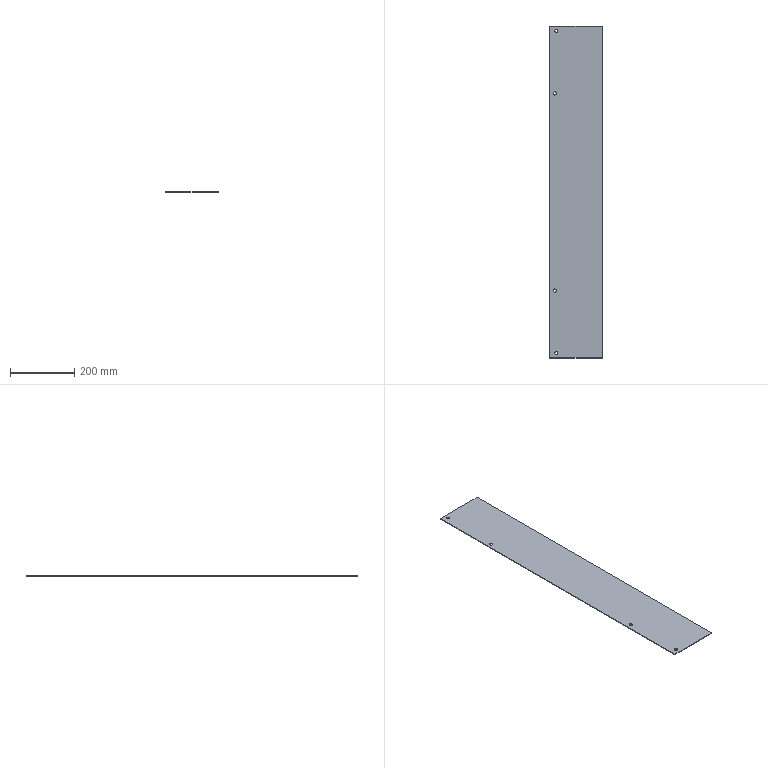Part | STEP file | 1 solid | 14 faces | box 162.5 x 1034 x 2 mm | volume 335422 mm3 | cylinder 8 | plane 6 | commonest cylinder face diameters 10 x8
STEP:
#1=CARTESIAN_POINT('',(0.,0.,0.));
#2=DIRECTION('',(0.,0.,1.));
#3=DIRECTION('',(1.,0.,0.));
#4=AXIS2_PLACEMENT_3D('',#1,#2,#3);
#5=CARTESIAN_POINT('',(-60.73,-722.451,2.));
#6=VERTEX_POINT('',#5);
#7=CARTESIAN_POINT('',(-60.73,-722.451,0.));
#8=VERTEX_POINT('',#7);
#9=CARTESIAN_POINT('',(-60.73,-722.451,2.));
#10=DIRECTION('',(0.,0.,-1.));
#11=VECTOR('',#10,1.);
#12=LINE('',#9,#11);
#13=CARTESIAN_POINT('',(-55.73,-722.451,2.));
#14=DIRECTION('',(0.,0.,-1.));
#15=DIRECTION('',(-1.,0.,0.));
#16=AXIS2_PLACEMENT_3D('',#13,#14,#15);
#17=CYLINDRICAL_SURFACE('',#16,5.);
#18=CARTESIAN_POINT('',(6.283,0.));
#19=DIRECTION('',(0.,1.));
#20=VECTOR('',#19,1.);
#21=LINE('',#18,#20);
#22=(GEOMETRIC_REPRESENTATION_CONTEXT(2)PARAMETRIC_REPRESENTATION_CONTEXT()REPRESENTATION_CONTEXT('',''));
#23=DEFINITIONAL_REPRESENTATION('',(#21),#22);
#24=PCURVE('',#17,#23);
#25=CARTESIAN_POINT('',(-55.73,-722.451,2.));
#26=DIRECTION('',(0.,0.,-1.));
#27=DIRECTION('',(-1.,0.,0.));
#28=AXIS2_PLACEMENT_3D('',#25,#26,#27);
#29=CYLINDRICAL_SURFACE('',#28,5.);
#30=CARTESIAN_POINT('',(0.,0.));
#31=DIRECTION('',(0.,1.));
#32=VECTOR('',#31,1.);
#33=LINE('',#30,#32);
#34=(GEOMETRIC_REPRESENTATION_CONTEXT(2)PARAMETRIC_REPRESENTATION_CONTEXT()REPRESENTATION_CONTEXT('',''));
#35=DEFINITIONAL_REPRESENTATION('',(#33),#34);
#36=PCURVE('',#29,#35);
#37=SURFACE_CURVE('',#12,(#24,#36),.PCURVE_S1.);
#38=EDGE_CURVE('',#6,#8,#37,.T.);
#39=ORIENTED_EDGE('',*,*,#38,.T.);
#40=CARTESIAN_POINT('',(-50.73,-722.451,0.));
#41=VERTEX_POINT('',#40);
#42=CARTESIAN_POINT('',(-55.73,-722.451,0.));
#43=DIRECTION('',(0.,0.,-1.));
#44=DIRECTION('',(-1.,0.,0.));
#45=AXIS2_PLACEMENT_3D('',#42,#43,#44);
#46=CIRCLE('',#45,5.);
#47=CARTESIAN_POINT('',(0.,2.));
#48=DIRECTION('',(1.,0.));
#49=VECTOR('',#48,1.);
#50=LINE('',#47,#49);
#51=(GEOMETRIC_REPRESENTATION_CONTEXT(2)PARAMETRIC_REPRESENTATION_CONTEXT()REPRESENTATION_CONTEXT('',''));
#52=DEFINITIONAL_REPRESENTATION('',(#50),#51);
#53=PCURVE('',#17,#52);
#54=CARTESIAN_POINT('',(10.52,-415.451,0.));
#55=DIRECTION('',(0.,0.,1.));
#56=DIRECTION('',(1.,0.,0.));
#57=AXIS2_PLACEMENT_3D('',#54,#55,#56);
#58=PLANE('',#57);
#59=CARTESIAN_POINT('',(-71.25,-307.));
#60=CARTESIAN_POINT('',(-71.25,-298.34));
#61=CARTESIAN_POINT('',(-63.75,-302.67));
#62=CARTESIAN_POINT('',(-56.25,-307.));
#63=CARTESIAN_POINT('',(-63.75,-311.33));
#64=CARTESIAN_POINT('',(-71.25,-315.66));
#65=CARTESIAN_POINT('',(-71.25,-307.));
#66=(BOUNDED_CURVE()B_SPLINE_CURVE(2,(#59,#60,#61,#62,#63,#64,#65),.UNSPECIFIED.,.T.,.F.)B_SPLINE_CURVE_WITH_KNOTS((1,2,2,2,2,1),(-2.094,0.,2.094,4.189,6.283,8.378),.UNSPECIFIED.)CURVE()GEOMETRIC_REPRESENTATION_ITEM()RATIONAL_B_SPLINE_CURVE((1.,0.5,1.,0.5,1.,0.5,1.))REPRESENTATION_ITEM(''));
#67=(GEOMETRIC_REPRESENTATION_CONTEXT(2)PARAMETRIC_REPRESENTATION_CONTEXT()REPRESENTATION_CONTEXT('',''));
#68=DEFINITIONAL_REPRESENTATION('',(#66),#67);
#69=PCURVE('',#58,#68);
#70=SURFACE_CURVE('',#46,(#53,#69),.PCURVE_S1.);
#71=EDGE_CURVE('',#41,#8,#70,.T.);
#72=ORIENTED_EDGE('',*,*,#71,.F.);
#73=CARTESIAN_POINT('',(-50.73,-722.451,2.));
#74=VERTEX_POINT('',#73);
#75=CARTESIAN_POINT('',(-50.73,-722.451,2.));
#76=DIRECTION('',(0.,0.,-1.));
#77=VECTOR('',#76,1.);
#78=LINE('',#75,#77);
#79=CARTESIAN_POINT('',(3.142,0.));
#80=DIRECTION('',(0.,1.));
#81=VECTOR('',#80,1.);
#82=LINE('',#79,#81);
#83=(GEOMETRIC_REPRESENTATION_CONTEXT(2)PARAMETRIC_REPRESENTATION_CONTEXT()REPRESENTATION_CONTEXT('',''));
#84=DEFINITIONAL_REPRESENTATION('',(#82),#83);
#85=PCURVE('',#17,#84);
#86=CARTESIAN_POINT('',(3.142,0.));
#87=DIRECTION('',(0.,1.));
#88=VECTOR('',#87,1.);
#89=LINE('',#86,#88);
#90=(GEOMETRIC_REPRESENTATION_CONTEXT(2)PARAMETRIC_REPRESENTATION_CONTEXT()REPRESENTATION_CONTEXT('',''));
#91=DEFINITIONAL_REPRESENTATION('',(#89),#90);
#92=PCURVE('',#29,#91);
#93=SURFACE_CURVE('',#78,(#85,#92),.PCURVE_S1.);
#94=EDGE_CURVE('',#74,#41,#93,.T.);
#95=ORIENTED_EDGE('',*,*,#94,.F.);
#96=CARTESIAN_POINT('',(-55.73,-722.451,2.));
#97=DIRECTION('',(0.,0.,-1.));
#98=DIRECTION('',(-1.,0.,0.));
#99=AXIS2_PLACEMENT_3D('',#96,#97,#98);
#100=CIRCLE('',#99,5.);
#101=CARTESIAN_POINT('',(0.,0.));
#102=DIRECTION('',(1.,0.));
#103=VECTOR('',#102,1.);
#104=LINE('',#101,#103);
#105=(GEOMETRIC_REPRESENTATION_CONTEXT(2)PARAMETRIC_REPRESENTATION_CONTEXT()REPRESENTATION_CONTEXT('',''));
#106=DEFINITIONAL_REPRESENTATION('',(#104),#105);
#107=PCURVE('',#17,#106);
#108=CARTESIAN_POINT('',(10.52,-415.451,2.));
#109=DIRECTION('',(0.,0.,1.));
#110=DIRECTION('',(1.,0.,0.));
#111=AXIS2_PLACEMENT_3D('',#108,#109,#110);
#112=PLANE('',#111);
#113=CARTESIAN_POINT('',(-71.25,-307.));
#114=CARTESIAN_POINT('',(-71.25,-298.34));
#115=CARTESIAN_POINT('',(-63.75,-302.67));
#116=CARTESIAN_POINT('',(-56.25,-307.));
#117=CARTESIAN_POINT('',(-63.75,-311.33));
#118=CARTESIAN_POINT('',(-71.25,-315.66));
#119=CARTESIAN_POINT('',(-71.25,-307.));
#120=(BOUNDED_CURVE()B_SPLINE_CURVE(2,(#113,#114,#115,#116,#117,#118,#119),.UNSPECIFIED.,.T.,.F.)B_SPLINE_CURVE_WITH_KNOTS((1,2,2,2,2,1),(-2.094,0.,2.094,4.189,6.283,8.378),.UNSPECIFIED.)CURVE()GEOMETRIC_REPRESENTATION_ITEM()RATIONAL_B_SPLINE_CURVE((1.,0.5,1.,0.5,1.,0.5,1.))REPRESENTATION_ITEM(''));
#121=(GEOMETRIC_REPRESENTATION_CONTEXT(2)PARAMETRIC_REPRESENTATION_CONTEXT()REPRESENTATION_CONTEXT('',''));
#122=DEFINITIONAL_REPRESENTATION('',(#120),#121);
#123=PCURVE('',#112,#122);
#124=SURFACE_CURVE('',#100,(#107,#123),.PCURVE_S1.);
#125=EDGE_CURVE('',#74,#6,#124,.T.);
#126=ORIENTED_EDGE('',*,*,#125,.T.);
#127=EDGE_LOOP('',(#39,#72,#95,#126));
#128=FACE_BOUND('',#127,.F.);
#129=ADVANCED_FACE('',(#128),#17,.F.);
#130=CARTESIAN_POINT('',(-60.73,-108.451,2.));
#131=VERTEX_POINT('',#130);
#132=CARTESIAN_POINT('',(-60.73,-108.451,0.));
#133=VERTEX_POINT('',#132);
#134=CARTESIAN_POINT('',(-60.73,-108.451,2.));
#135=DIRECTION('',(0.,0.,-1.));
#136=VECTOR('',#135,1.);
#137=LINE('',#134,#136);
#138=CARTESIAN_POINT('',(-55.73,-108.451,2.));
#139=DIRECTION('',(0.,0.,-1.));
#140=DIRECTION('',(-1.,0.,0.));
#141=AXIS2_PLACEMENT_3D('',#138,#139,#140);
#142=CYLINDRICAL_SURFACE('',#141,5.);
#143=CARTESIAN_POINT('',(6.283,0.));
#144=DIRECTION('',(0.,1.));
#145=VECTOR('',#144,1.);
#146=LINE('',#143,#145);
#147=(GEOMETRIC_REPRESENTATION_CONTEXT(2)PARAMETRIC_REPRESENTATION_CONTEXT()REPRESENTATION_CONTEXT('',''));
#148=DEFINITIONAL_REPRESENTATION('',(#146),#147);
#149=PCURVE('',#142,#148);
#150=CARTESIAN_POINT('',(-55.73,-108.451,2.));
#151=DIRECTION('',(0.,0.,-1.));
#152=DIRECTION('',(-1.,0.,0.));
#153=AXIS2_PLACEMENT_3D('',#150,#151,#152);
#154=CYLINDRICAL_SURFACE('',#153,5.);
#155=CARTESIAN_POINT('',(0.,0.));
#156=DIRECTION('',(0.,1.));
#157=VECTOR('',#156,1.);
#158=LINE('',#155,#157);
#159=(GEOMETRIC_REPRESENTATION_CONTEXT(2)PARAMETRIC_REPRESENTATION_CONTEXT()REPRESENTATION_CONTEXT('',''));
#160=DEFINITIONAL_REPRESENTATION('',(#158),#159);
#161=PCURVE('',#154,#160);
#162=SURFACE_CURVE('',#137,(#149,#161),.PCURVE_S1.);
#163=EDGE_CURVE('',#131,#133,#162,.T.);
#164=ORIENTED_EDGE('',*,*,#163,.T.);
#165=CARTESIAN_POINT('',(-50.73,-108.451,0.));
#166=VERTEX_POINT('',#165);
#167=CARTESIAN_POINT('',(-55.73,-108.451,0.));
#168=DIRECTION('',(0.,0.,-1.));
#169=DIRECTION('',(-1.,0.,0.));
#170=AXIS2_PLACEMENT_3D('',#167,#168,#169);
#171=CIRCLE('',#170,5.);
#172=CARTESIAN_POINT('',(0.,2.));
#173=DIRECTION('',(1.,0.));
#174=VECTOR('',#173,1.);
#175=LINE('',#172,#174);
#176=(GEOMETRIC_REPRESENTATION_CONTEXT(2)PARAMETRIC_REPRESENTATION_CONTEXT()REPRESENTATION_CONTEXT('',''));
#177=DEFINITIONAL_REPRESENTATION('',(#175),#176);
#178=PCURVE('',#142,#177);
#179=CARTESIAN_POINT('',(-71.25,307.));
#180=CARTESIAN_POINT('',(-71.25,315.66));
#181=CARTESIAN_POINT('',(-63.75,311.33));
#182=CARTESIAN_POINT('',(-56.25,307.));
#183=CARTESIAN_POINT('',(-63.75,302.67));
#184=CARTESIAN_POINT('',(-71.25,298.34));
#185=CARTESIAN_POINT('',(-71.25,307.));
#186=(BOUNDED_CURVE()B_SPLINE_CURVE(2,(#179,#180,#181,#182,#183,#184,#185),.UNSPECIFIED.,.T.,.F.)B_SPLINE_CURVE_WITH_KNOTS((1,2,2,2,2,1),(-2.094,0.,2.094,4.189,6.283,8.378),.UNSPECIFIED.)CURVE()GEOMETRIC_REPRESENTATION_ITEM()RATIONAL_B_SPLINE_CURVE((1.,0.5,1.,0.5,1.,0.5,1.))REPRESENTATION_ITEM(''));
#187=(GEOMETRIC_REPRESENTATION_CONTEXT(2)PARAMETRIC_REPRESENTATION_CONTEXT()REPRESENTATION_CONTEXT('',''));
#188=DEFINITIONAL_REPRESENTATION('',(#186),#187);
#189=PCURVE('',#58,#188);
#190=SURFACE_CURVE('',#171,(#178,#189),.PCURVE_S1.);
#191=EDGE_CURVE('',#166,#133,#190,.T.);
#192=ORIENTED_EDGE('',*,*,#191,.F.);
#193=CARTESIAN_POINT('',(-50.73,-108.451,2.));
#194=VERTEX_POINT('',#193);
#195=CARTESIAN_POINT('',(-50.73,-108.451,2.));
#196=DIRECTION('',(0.,0.,-1.));
#197=VECTOR('',#196,1.);
#198=LINE('',#195,#197);
#199=CARTESIAN_POINT('',(3.142,0.));
#200=DIRECTION('',(0.,1.));
#201=VECTOR('',#200,1.);
#202=LINE('',#199,#201);
#203=(GEOMETRIC_REPRESENTATION_CONTEXT(2)PARAMETRIC_REPRESENTATION_CONTEXT()REPRESENTATION_CONTEXT('',''));
#204=DEFINITIONAL_REPRESENTATION('',(#202),#203);
#205=PCURVE('',#142,#204);
#206=CARTESIAN_POINT('',(3.142,0.));
#207=DIRECTION('',(0.,1.));
#208=VECTOR('',#207,1.);
#209=LINE('',#206,#208);
#210=(GEOMETRIC_REPRESENTATION_CONTEXT(2)PARAMETRIC_REPRESENTATION_CONTEXT()REPRESENTATION_CONTEXT('',''));
#211=DEFINITIONAL_REPRESENTATION('',(#209),#210);
#212=PCURVE('',#154,#211);
#213=SURFACE_CURVE('',#198,(#205,#212),.PCURVE_S1.);
#214=EDGE_CURVE('',#194,#166,#213,.T.);
#215=ORIENTED_EDGE('',*,*,#214,.F.);
#216=CARTESIAN_POINT('',(-55.73,-108.451,2.));
#217=DIRECTION('',(0.,0.,-1.));
#218=DIRECTION('',(-1.,0.,0.));
#219=AXIS2_PLACEMENT_3D('',#216,#217,#218);
#220=CIRCLE('',#219,5.);
#221=CARTESIAN_POINT('',(0.,0.));
#222=DIRECTION('',(1.,0.));
#223=VECTOR('',#222,1.);
#224=LINE('',#221,#223);
#225=(GEOMETRIC_REPRESENTATION_CONTEXT(2)PARAMETRIC_REPRESENTATION_CONTEXT()REPRESENTATION_CONTEXT('',''));
#226=DEFINITIONAL_REPRESENTATION('',(#224),#225);
#227=PCURVE('',#142,#226);
#228=CARTESIAN_POINT('',(-71.25,307.));
#229=CARTESIAN_POINT('',(-71.25,315.66));
#230=CARTESIAN_POINT('',(-63.75,311.33));
#231=CARTESIAN_POINT('',(-56.25,307.));
#232=CARTESIAN_POINT('',(-63.75,302.67));
#233=CARTESIAN_POINT('',(-71.25,298.34));
#234=CARTESIAN_POINT('',(-71.25,307.));
#235=(BOUNDED_CURVE()B_SPLINE_CURVE(2,(#228,#229,#230,#231,#232,#233,#234),.UNSPECIFIED.,.T.,.F.)B_SPLINE_CURVE_WITH_KNOTS((1,2,2,2,2,1),(-2.094,0.,2.094,4.189,6.283,8.378),.UNSPECIFIED.)CURVE()GEOMETRIC_REPRESENTATION_ITEM()RATIONAL_B_SPLINE_CURVE((1.,0.5,1.,0.5,1.,0.5,1.))REPRESENTATION_ITEM(''));
#236=(GEOMETRIC_REPRESENTATION_CONTEXT(2)PARAMETRIC_REPRESENTATION_CONTEXT()REPRESENTATION_CONTEXT('',''));
#237=DEFINITIONAL_REPRESENTATION('',(#235),#236);
#238=PCURVE('',#112,#237);
#239=SURFACE_CURVE('',#220,(#227,#238),.PCURVE_S1.);
#240=EDGE_CURVE('',#194,#131,#239,.T.);
#241=ORIENTED_EDGE('',*,*,#240,.T.);
#242=EDGE_LOOP('',(#164,#192,#215,#241));
#243=FACE_BOUND('',#242,.F.);
#244=ADVANCED_FACE('',(#243),#142,.F.);
#245=CARTESIAN_POINT('',(-55.73,-917.451,2.));
#246=VERTEX_POINT('',#245);
#247=CARTESIAN_POINT('',(-55.73,-917.451,0.));
#248=VERTEX_POINT('',#247);
#249=CARTESIAN_POINT('',(-55.73,-917.451,2.));
#250=DIRECTION('',(0.,0.,-1.));
#251=VECTOR('',#250,1.);
#252=LINE('',#249,#251);
#253=CARTESIAN_POINT('',(-50.73,-917.451,2.));
#254=DIRECTION('',(0.,0.,-1.));
#255=DIRECTION('',(-1.,0.,0.));
#256=AXIS2_PLACEMENT_3D('',#253,#254,#255);
#257=CYLINDRICAL_SURFACE('',#256,5.);
#258=CARTESIAN_POINT('',(6.283,0.));
#259=DIRECTION('',(0.,1.));
#260=VECTOR('',#259,1.);
#261=LINE('',#258,#260);
#262=(GEOMETRIC_REPRESENTATION_CONTEXT(2)PARAMETRIC_REPRESENTATION_CONTEXT()REPRESENTATION_CONTEXT('',''));
#263=DEFINITIONAL_REPRESENTATION('',(#261),#262);
#264=PCURVE('',#257,#263);
#265=CARTESIAN_POINT('',(-50.73,-917.451,2.));
#266=DIRECTION('',(0.,0.,-1.));
#267=DIRECTION('',(-1.,0.,0.));
#268=AXIS2_PLACEMENT_3D('',#265,#266,#267);
#269=CYLINDRICAL_SURFACE('',#268,5.);
#270=CARTESIAN_POINT('',(0.,0.));
#271=DIRECTION('',(0.,1.));
#272=VECTOR('',#271,1.);
#273=LINE('',#270,#272);
#274=(GEOMETRIC_REPRESENTATION_CONTEXT(2)PARAMETRIC_REPRESENTATION_CONTEXT()REPRESENTATION_CONTEXT('',''));
#275=DEFINITIONAL_REPRESENTATION('',(#273),#274);
#276=PCURVE('',#269,#275);
#277=SURFACE_CURVE('',#252,(#264,#276),.PCURVE_S1.);
#278=EDGE_CURVE('',#246,#248,#277,.T.);
#279=ORIENTED_EDGE('',*,*,#278,.T.);
#280=CARTESIAN_POINT('',(-45.73,-917.451,0.));
#281=VERTEX_POINT('',#280);
#282=CARTESIAN_POINT('',(-50.73,-917.451,0.));
#283=DIRECTION('',(0.,0.,-1.));
#284=DIRECTION('',(-1.,0.,0.));
#285=AXIS2_PLACEMENT_3D('',#282,#283,#284);
#286=CIRCLE('',#285,5.);
#287=CARTESIAN_POINT('',(0.,2.));
#288=DIRECTION('',(1.,0.));
#289=VECTOR('',#288,1.);
#290=LINE('',#287,#289);
#291=(GEOMETRIC_REPRESENTATION_CONTEXT(2)PARAMETRIC_REPRESENTATION_CONTEXT()REPRESENTATION_CONTEXT('',''));
#292=DEFINITIONAL_REPRESENTATION('',(#290),#291);
#293=PCURVE('',#257,#292);
#294=CARTESIAN_POINT('',(-66.25,-502.));
#295=CARTESIAN_POINT('',(-66.25,-493.34));
#296=CARTESIAN_POINT('',(-58.75,-497.67));
#297=CARTESIAN_POINT('',(-51.25,-502.));
#298=CARTESIAN_POINT('',(-58.75,-506.33));
#299=CARTESIAN_POINT('',(-66.25,-510.66));
#300=CARTESIAN_POINT('',(-66.25,-502.));
#301=(BOUNDED_CURVE()B_SPLINE_CURVE(2,(#294,#295,#296,#297,#298,#299,#300),.UNSPECIFIED.,.T.,.F.)B_SPLINE_CURVE_WITH_KNOTS((1,2,2,2,2,1),(-2.094,0.,2.094,4.189,6.283,8.378),.UNSPECIFIED.)CURVE()GEOMETRIC_REPRESENTATION_ITEM()RATIONAL_B_SPLINE_CURVE((1.,0.5,1.,0.5,1.,0.5,1.))REPRESENTATION_ITEM(''));
#302=(GEOMETRIC_REPRESENTATION_CONTEXT(2)PARAMETRIC_REPRESENTATION_CONTEXT()REPRESENTATION_CONTEXT('',''));
#303=DEFINITIONAL_REPRESENTATION('',(#301),#302);
#304=PCURVE('',#58,#303);
#305=SURFACE_CURVE('',#286,(#293,#304),.PCURVE_S1.);
#306=EDGE_CURVE('',#281,#248,#305,.T.);
#307=ORIENTED_EDGE('',*,*,#306,.F.);
#308=CARTESIAN_POINT('',(-45.73,-917.451,2.));
#309=VERTEX_POINT('',#308);
#310=CARTESIAN_POINT('',(-45.73,-917.451,2.));
#311=DIRECTION('',(0.,0.,-1.));
#312=VECTOR('',#311,1.);
#313=LINE('',#310,#312);
#314=CARTESIAN_POINT('',(3.142,0.));
#315=DIRECTION('',(0.,1.));
#316=VECTOR('',#315,1.);
#317=LINE('',#314,#316);
#318=(GEOMETRIC_REPRESENTATION_CONTEXT(2)PARAMETRIC_REPRESENTATION_CONTEXT()REPRESENTATION_CONTEXT('',''));
#319=DEFINITIONAL_REPRESENTATION('',(#317),#318);
#320=PCURVE('',#257,#319);
#321=CARTESIAN_POINT('',(3.142,0.));
#322=DIRECTION('',(0.,1.));
#323=VECTOR('',#322,1.);
#324=LINE('',#321,#323);
#325=(GEOMETRIC_REPRESENTATION_CONTEXT(2)PARAMETRIC_REPRESENTATION_CONTEXT()REPRESENTATION_CONTEXT('',''));
#326=DEFINITIONAL_REPRESENTATION('',(#324),#325);
#327=PCURVE('',#269,#326);
#328=SURFACE_CURVE('',#313,(#320,#327),.PCURVE_S1.);
#329=EDGE_CURVE('',#309,#281,#328,.T.);
#330=ORIENTED_EDGE('',*,*,#329,.F.);
#331=CARTESIAN_POINT('',(-50.73,-917.451,2.));
#332=DIRECTION('',(0.,0.,-1.));
#333=DIRECTION('',(-1.,0.,0.));
#334=AXIS2_PLACEMENT_3D('',#331,#332,#333);
#335=CIRCLE('',#334,5.);
#336=CARTESIAN_POINT('',(0.,0.));
#337=DIRECTION('',(1.,0.));
#338=VECTOR('',#337,1.);
#339=LINE('',#336,#338);
#340=(GEOMETRIC_REPRESENTATION_CONTEXT(2)PARAMETRIC_REPRESENTATION_CONTEXT()REPRESENTATION_CONTEXT('',''));
#341=DEFINITIONAL_REPRESENTATION('',(#339),#340);
#342=PCURVE('',#257,#341);
#343=CARTESIAN_POINT('',(-66.25,-502.));
#344=CARTESIAN_POINT('',(-66.25,-493.34));
#345=CARTESIAN_POINT('',(-58.75,-497.67));
#346=CARTESIAN_POINT('',(-51.25,-502.));
#347=CARTESIAN_POINT('',(-58.75,-506.33));
#348=CARTESIAN_POINT('',(-66.25,-510.66));
#349=CARTESIAN_POINT('',(-66.25,-502.));
#350=(BOUNDED_CURVE()B_SPLINE_CURVE(2,(#343,#344,#345,#346,#347,#348,#349),.UNSPECIFIED.,.T.,.F.)B_SPLINE_CURVE_WITH_KNOTS((1,2,2,2,2,1),(-2.094,0.,2.094,4.189,6.283,8.378),.UNSPECIFIED.)CURVE()GEOMETRIC_REPRESENTATION_ITEM()RATIONAL_B_SPLINE_CURVE((1.,0.5,1.,0.5,1.,0.5,1.))REPRESENTATION_ITEM(''));
#351=(GEOMETRIC_REPRESENTATION_CONTEXT(2)PARAMETRIC_REPRESENTATION_CONTEXT()REPRESENTATION_CONTEXT('',''));
#352=DEFINITIONAL_REPRESENTATION('',(#350),#351);
#353=PCURVE('',#112,#352);
#354=SURFACE_CURVE('',#335,(#342,#353),.PCURVE_S1.);
#355=EDGE_CURVE('',#309,#246,#354,.T.);
#356=ORIENTED_EDGE('',*,*,#355,.T.);
#357=EDGE_LOOP('',(#279,#307,#330,#356));
#358=FACE_BOUND('',#357,.F.);
#359=ADVANCED_FACE('',(#358),#257,.F.);
#360=CARTESIAN_POINT('',(-55.73,86.549,2.));
#361=VERTEX_POINT('',#360);
#362=CARTESIAN_POINT('',(-55.73,86.549,0.));
#363=VERTEX_POINT('',#362);
#364=CARTESIAN_POINT('',(-55.73,86.549,2.));
#365=DIRECTION('',(0.,0.,-1.));
#366=VECTOR('',#365,1.);
#367=LINE('',#364,#366);
#368=CARTESIAN_POINT('',(-50.73,86.549,2.));
#369=DIRECTION('',(0.,0.,-1.));
#370=DIRECTION('',(-1.,0.,0.));
#371=AXIS2_PLACEMENT_3D('',#368,#369,#370);
#372=CYLINDRICAL_SURFACE('',#371,5.);
#373=CARTESIAN_POINT('',(6.283,0.));
#374=DIRECTION('',(0.,1.));
#375=VECTOR('',#374,1.);
#376=LINE('',#373,#375);
#377=(GEOMETRIC_REPRESENTATION_CONTEXT(2)PARAMETRIC_REPRESENTATION_CONTEXT()REPRESENTATION_CONTEXT('',''));
#378=DEFINITIONAL_REPRESENTATION('',(#376),#377);
#379=PCURVE('',#372,#378);
#380=CARTESIAN_POINT('',(-50.73,86.549,2.));
#381=DIRECTION('',(0.,0.,-1.));
#382=DIRECTION('',(-1.,0.,0.));
#383=AXIS2_PLACEMENT_3D('',#380,#381,#382);
#384=CYLINDRICAL_SURFACE('',#383,5.);
#385=CARTESIAN_POINT('',(0.,0.));
#386=DIRECTION('',(0.,1.));
#387=VECTOR('',#386,1.);
#388=LINE('',#385,#387);
#389=(GEOMETRIC_REPRESENTATION_CONTEXT(2)PARAMETRIC_REPRESENTATION_CONTEXT()REPRESENTATION_CONTEXT('',''));
#390=DEFINITIONAL_REPRESENTATION('',(#388),#389);
#391=PCURVE('',#384,#390);
#392=SURFACE_CURVE('',#367,(#379,#391),.PCURVE_S1.);
#393=EDGE_CURVE('',#361,#363,#392,.T.);
#394=ORIENTED_EDGE('',*,*,#393,.T.);
#395=CARTESIAN_POINT('',(-45.73,86.549,0.));
#396=VERTEX_POINT('',#395);
#397=CARTESIAN_POINT('',(-50.73,86.549,0.));
#398=DIRECTION('',(0.,0.,-1.));
#399=DIRECTION('',(-1.,0.,0.));
#400=AXIS2_PLACEMENT_3D('',#397,#398,#399);
#401=CIRCLE('',#400,5.);
#402=CARTESIAN_POINT('',(0.,2.));
#403=DIRECTION('',(1.,0.));
#404=VECTOR('',#403,1.);
#405=LINE('',#402,#404);
#406=(GEOMETRIC_REPRESENTATION_CONTEXT(2)PARAMETRIC_REPRESENTATION_CONTEXT()REPRESENTATION_CONTEXT('',''));
#407=DEFINITIONAL_REPRESENTATION('',(#405),#406);
#408=PCURVE('',#372,#407);
#409=CARTESIAN_POINT('',(-66.25,502.));
#410=CARTESIAN_POINT('',(-66.25,510.66));
#411=CARTESIAN_POINT('',(-58.75,506.33));
#412=CARTESIAN_POINT('',(-51.25,502.));
#413=CARTESIAN_POINT('',(-58.75,497.67));
#414=CARTESIAN_POINT('',(-66.25,493.34));
#415=CARTESIAN_POINT('',(-66.25,502.));
#416=(BOUNDED_CURVE()B_SPLINE_CURVE(2,(#409,#410,#411,#412,#413,#414,#415),.UNSPECIFIED.,.T.,.F.)B_SPLINE_CURVE_WITH_KNOTS((1,2,2,2,2,1),(-2.094,0.,2.094,4.189,6.283,8.378),.UNSPECIFIED.)CURVE()GEOMETRIC_REPRESENTATION_ITEM()RATIONAL_B_SPLINE_CURVE((1.,0.5,1.,0.5,1.,0.5,1.))REPRESENTATION_ITEM(''));
#417=(GEOMETRIC_REPRESENTATION_CONTEXT(2)PARAMETRIC_REPRESENTATION_CONTEXT()REPRESENTATION_CONTEXT('',''));
#418=DEFINITIONAL_REPRESENTATION('',(#416),#417);
#419=PCURVE('',#58,#418);
#420=SURFACE_CURVE('',#401,(#408,#419),.PCURVE_S1.);
#421=EDGE_CURVE('',#396,#363,#420,.T.);
#422=ORIENTED_EDGE('',*,*,#421,.F.);
#423=CARTESIAN_POINT('',(-45.73,86.549,2.));
#424=VERTEX_POINT('',#423);
#425=CARTESIAN_POINT('',(-45.73,86.549,2.));
#426=DIRECTION('',(0.,0.,-1.));
#427=VECTOR('',#426,1.);
#428=LINE('',#425,#427);
#429=CARTESIAN_POINT('',(3.142,0.));
#430=DIRECTION('',(0.,1.));
#431=VECTOR('',#430,1.);
#432=LINE('',#429,#431);
#433=(GEOMETRIC_REPRESENTATION_CONTEXT(2)PARAMETRIC_REPRESENTATION_CONTEXT()REPRESENTATION_CONTEXT('',''));
#434=DEFINITIONAL_REPRESENTATION('',(#432),#433);
#435=PCURVE('',#372,#434);
#436=CARTESIAN_POINT('',(3.142,0.));
#437=DIRECTION('',(0.,1.));
#438=VECTOR('',#437,1.);
#439=LINE('',#436,#438);
#440=(GEOMETRIC_REPRESENTATION_CONTEXT(2)PARAMETRIC_REPRESENTATION_CONTEXT()REPRESENTATION_CONTEXT('',''));
#441=DEFINITIONAL_REPRESENTATION('',(#439),#440);
#442=PCURVE('',#384,#441);
#443=SURFACE_CURVE('',#428,(#435,#442),.PCURVE_S1.);
#444=EDGE_CURVE('',#424,#396,#443,.T.);
#445=ORIENTED_EDGE('',*,*,#444,.F.);
#446=CARTESIAN_POINT('',(-50.73,86.549,2.));
#447=DIRECTION('',(0.,0.,-1.));
#448=DIRECTION('',(-1.,0.,0.));
#449=AXIS2_PLACEMENT_3D('',#446,#447,#448);
#450=CIRCLE('',#449,5.);
#451=CARTESIAN_POINT('',(0.,0.));
#452=DIRECTION('',(1.,0.));
#453=VECTOR('',#452,1.);
#454=LINE('',#451,#453);
#455=(GEOMETRIC_REPRESENTATION_CONTEXT(2)PARAMETRIC_REPRESENTATION_CONTEXT()REPRESENTATION_CONTEXT('',''));
#456=DEFINITIONAL_REPRESENTATION('',(#454),#455);
#457=PCURVE('',#372,#456);
#458=CARTESIAN_POINT('',(-66.25,502.));
#459=CARTESIAN_POINT('',(-66.25,510.66));
#460=CARTESIAN_POINT('',(-58.75,506.33));
#461=CARTESIAN_POINT('',(-51.25,502.));
#462=CARTESIAN_POINT('',(-58.75,497.67));
#463=CARTESIAN_POINT('',(-66.25,493.34));
#464=CARTESIAN_POINT('',(-66.25,502.));
#465=(BOUNDED_CURVE()B_SPLINE_CURVE(2,(#458,#459,#460,#461,#462,#463,#464),.UNSPECIFIED.,.T.,.F.)B_SPLINE_CURVE_WITH_KNOTS((1,2,2,2,2,1),(-2.094,0.,2.094,4.189,6.283,8.378),.UNSPECIFIED.)CURVE()GEOMETRIC_REPRESENTATION_ITEM()RATIONAL_B_SPLINE_CURVE((1.,0.5,1.,0.5,1.,0.5,1.))REPRESENTATION_ITEM(''));
#466=(GEOMETRIC_REPRESENTATION_CONTEXT(2)PARAMETRIC_REPRESENTATION_CONTEXT()REPRESENTATION_CONTEXT('',''));
#467=DEFINITIONAL_REPRESENTATION('',(#465),#466);
#468=PCURVE('',#112,#467);
#469=SURFACE_CURVE('',#450,(#457,#468),.PCURVE_S1.);
#470=EDGE_CURVE('',#424,#361,#469,.T.);
#471=ORIENTED_EDGE('',*,*,#470,.T.);
#472=EDGE_LOOP('',(#394,#422,#445,#471));
#473=FACE_BOUND('',#472,.F.);
#474=ADVANCED_FACE('',(#473),#372,.F.);
#475=CARTESIAN_POINT('',(91.77,-932.451,0.));
#476=VERTEX_POINT('',#475);
#477=CARTESIAN_POINT('',(91.77,101.549,0.));
#478=VERTEX_POINT('',#477);
#479=CARTESIAN_POINT('',(91.77,-415.451,0.));
#480=DIRECTION('',(0.,1.,0.));
#481=VECTOR('',#480,1.);
#482=LINE('',#479,#481);
#483=CARTESIAN_POINT('',(81.25,0.));
#484=DIRECTION('',(0.,1.));
#485=VECTOR('',#484,1.);
#486=LINE('',#483,#485);
#487=(GEOMETRIC_REPRESENTATION_CONTEXT(2)PARAMETRIC_REPRESENTATION_CONTEXT()REPRESENTATION_CONTEXT('',''));
#488=DEFINITIONAL_REPRESENTATION('',(#486),#487);
#489=PCURVE('',#58,#488);
#490=CARTESIAN_POINT('',(91.77,-932.451,0.));
#491=DIRECTION('',(1.,0.,0.));
#492=DIRECTION('',(0.,1.,0.));
#493=AXIS2_PLACEMENT_3D('',#490,#491,#492);
#494=PLANE('',#493);
#495=CARTESIAN_POINT('',(517.,0.));
#496=DIRECTION('',(1.,0.));
#497=VECTOR('',#496,1.);
#498=LINE('',#495,#497);
#499=(GEOMETRIC_REPRESENTATION_CONTEXT(2)PARAMETRIC_REPRESENTATION_CONTEXT()REPRESENTATION_CONTEXT('',''));
#500=DEFINITIONAL_REPRESENTATION('',(#498),#499);
#501=PCURVE('',#494,#500);
#502=SURFACE_CURVE('',#482,(#489,#501),.PCURVE_S1.);
#503=EDGE_CURVE('',#476,#478,#502,.T.);
#504=ORIENTED_EDGE('',*,*,#503,.F.);
#505=CARTESIAN_POINT('',(-70.73,-932.451,0.));
#506=VERTEX_POINT('',#505);
#507=CARTESIAN_POINT('',(10.52,-932.451,0.));
#508=DIRECTION('',(1.,0.,0.));
#509=VECTOR('',#508,1.);
#510=LINE('',#507,#509);
#511=CARTESIAN_POINT('',(0.,-517.));
#512=DIRECTION('',(1.,0.));
#513=VECTOR('',#512,1.);
#514=LINE('',#511,#513);
#515=(GEOMETRIC_REPRESENTATION_CONTEXT(2)PARAMETRIC_REPRESENTATION_CONTEXT()REPRESENTATION_CONTEXT('',''));
#516=DEFINITIONAL_REPRESENTATION('',(#514),#515);
#517=PCURVE('',#58,#516);
#518=CARTESIAN_POINT('',(-70.73,-932.451,0.));
#519=DIRECTION('',(0.,-1.,0.));
#520=DIRECTION('',(0.,0.,-1.));
#521=AXIS2_PLACEMENT_3D('',#518,#519,#520);
#522=PLANE('',#521);
#523=CARTESIAN_POINT('',(0.,81.25));
#524=DIRECTION('',(0.,1.));
#525=VECTOR('',#524,1.);
#526=LINE('',#523,#525);
#527=(GEOMETRIC_REPRESENTATION_CONTEXT(2)PARAMETRIC_REPRESENTATION_CONTEXT()REPRESENTATION_CONTEXT('',''));
#528=DEFINITIONAL_REPRESENTATION('',(#526),#527);
#529=PCURVE('',#522,#528);
#530=SURFACE_CURVE('',#510,(#517,#529),.PCURVE_S1.);
#531=EDGE_CURVE('',#506,#476,#530,.T.);
#532=ORIENTED_EDGE('',*,*,#531,.F.);
#533=CARTESIAN_POINT('',(-70.73,101.549,0.));
#534=VERTEX_POINT('',#533);
#535=CARTESIAN_POINT('',(-70.73,-415.451,0.));
#536=DIRECTION('',(0.,-1.,0.));
#537=VECTOR('',#536,1.);
#538=LINE('',#535,#537);
#539=CARTESIAN_POINT('',(-81.25,0.));
#540=DIRECTION('',(0.,-1.));
#541=VECTOR('',#540,1.);
#542=LINE('',#539,#541);
#543=(GEOMETRIC_REPRESENTATION_CONTEXT(2)PARAMETRIC_REPRESENTATION_CONTEXT()REPRESENTATION_CONTEXT('',''));
#544=DEFINITIONAL_REPRESENTATION('',(#542),#543);
#545=PCURVE('',#58,#544);
#546=CARTESIAN_POINT('',(-70.73,101.549,0.));
#547=DIRECTION('',(-1.,0.,0.));
#548=DIRECTION('',(0.,-1.,0.));
#549=AXIS2_PLACEMENT_3D('',#546,#547,#548);
#550=PLANE('',#549);
#551=CARTESIAN_POINT('',(517.,0.));
#552=DIRECTION('',(1.,0.));
#553=VECTOR('',#552,1.);
#554=LINE('',#551,#553);
#555=(GEOMETRIC_REPRESENTATION_CONTEXT(2)PARAMETRIC_REPRESENTATION_CONTEXT()REPRESENTATION_CONTEXT('',''));
#556=DEFINITIONAL_REPRESENTATION('',(#554),#555);
#557=PCURVE('',#550,#556);
#558=SURFACE_CURVE('',#538,(#545,#557),.PCURVE_S1.);
#559=EDGE_CURVE('',#534,#506,#558,.T.);
#560=ORIENTED_EDGE('',*,*,#559,.F.);
#561=CARTESIAN_POINT('',(10.52,101.549,0.));
#562=DIRECTION('',(-1.,0.,0.));
#563=VECTOR('',#562,1.);
#564=LINE('',#561,#563);
#565=CARTESIAN_POINT('',(0.,517.));
#566=DIRECTION('',(-1.,0.));
#567=VECTOR('',#566,1.);
#568=LINE('',#565,#567);
#569=(GEOMETRIC_REPRESENTATION_CONTEXT(2)PARAMETRIC_REPRESENTATION_CONTEXT()REPRESENTATION_CONTEXT('',''));
#570=DEFINITIONAL_REPRESENTATION('',(#568),#569);
#571=PCURVE('',#58,#570);
#572=CARTESIAN_POINT('',(91.77,101.549,0.));
#573=DIRECTION('',(0.,1.,0.));
#574=DIRECTION('',(0.,0.,1.));
#575=AXIS2_PLACEMENT_3D('',#572,#573,#574);
#576=PLANE('',#575);
#577=CARTESIAN_POINT('',(0.,-81.25));
#578=DIRECTION('',(0.,-1.));
#579=VECTOR('',#578,1.);
#580=LINE('',#577,#579);
#581=(GEOMETRIC_REPRESENTATION_CONTEXT(2)PARAMETRIC_REPRESENTATION_CONTEXT()REPRESENTATION_CONTEXT('',''));
#582=DEFINITIONAL_REPRESENTATION('',(#580),#581);
#583=PCURVE('',#576,#582);
#584=SURFACE_CURVE('',#564,(#571,#583),.PCURVE_S1.);
#585=EDGE_CURVE('',#478,#534,#584,.T.);
#586=ORIENTED_EDGE('',*,*,#585,.F.);
#587=EDGE_LOOP('',(#504,#532,#560,#586));
#588=FACE_BOUND('',#587,.T.);
#589=CARTESIAN_POINT('',(-55.73,-722.451,0.));
#590=DIRECTION('',(0.,0.,-1.));
#591=DIRECTION('',(-1.,0.,0.));
#592=AXIS2_PLACEMENT_3D('',#589,#590,#591);
#593=CIRCLE('',#592,5.);
#594=CARTESIAN_POINT('',(-71.25,-307.));
#595=CARTESIAN_POINT('',(-71.25,-298.34));
#596=CARTESIAN_POINT('',(-63.75,-302.67));
#597=CARTESIAN_POINT('',(-56.25,-307.));
#598=CARTESIAN_POINT('',(-63.75,-311.33));
#599=CARTESIAN_POINT('',(-71.25,-315.66));
#600=CARTESIAN_POINT('',(-71.25,-307.));
#601=(BOUNDED_CURVE()B_SPLINE_CURVE(2,(#594,#595,#596,#597,#598,#599,#600),.UNSPECIFIED.,.T.,.F.)B_SPLINE_CURVE_WITH_KNOTS((1,2,2,2,2,1),(-2.094,0.,2.094,4.189,6.283,8.378),.UNSPECIFIED.)CURVE()GEOMETRIC_REPRESENTATION_ITEM()RATIONAL_B_SPLINE_CURVE((1.,0.5,1.,0.5,1.,0.5,1.))REPRESENTATION_ITEM(''));
#602=(GEOMETRIC_REPRESENTATION_CONTEXT(2)PARAMETRIC_REPRESENTATION_CONTEXT()REPRESENTATION_CONTEXT('',''));
#603=DEFINITIONAL_REPRESENTATION('',(#601),#602);
#604=PCURVE('',#58,#603);
#605=CARTESIAN_POINT('',(0.,2.));
#606=DIRECTION('',(1.,0.));
#607=VECTOR('',#606,1.);
#608=LINE('',#605,#607);
#609=(GEOMETRIC_REPRESENTATION_CONTEXT(2)PARAMETRIC_REPRESENTATION_CONTEXT()REPRESENTATION_CONTEXT('',''));
#610=DEFINITIONAL_REPRESENTATION('',(#608),#609);
#611=PCURVE('',#29,#610);
#612=SURFACE_CURVE('',#593,(#604,#611),.PCURVE_S1.);
#613=EDGE_CURVE('',#8,#41,#612,.T.);
#614=ORIENTED_EDGE('',*,*,#613,.F.);
#615=ORIENTED_EDGE('',*,*,#71,.F.);
#616=EDGE_LOOP('',(#614,#615));
#617=FACE_BOUND('',#616,.T.);
#618=CARTESIAN_POINT('',(-55.73,-108.451,0.));
#619=DIRECTION('',(0.,0.,-1.));
#620=DIRECTION('',(-1.,0.,0.));
#621=AXIS2_PLACEMENT_3D('',#618,#619,#620);
#622=CIRCLE('',#621,5.);
#623=CARTESIAN_POINT('',(-71.25,307.));
#624=CARTESIAN_POINT('',(-71.25,315.66));
#625=CARTESIAN_POINT('',(-63.75,311.33));
#626=CARTESIAN_POINT('',(-56.25,307.));
#627=CARTESIAN_POINT('',(-63.75,302.67));
#628=CARTESIAN_POINT('',(-71.25,298.34));
#629=CARTESIAN_POINT('',(-71.25,307.));
#630=(BOUNDED_CURVE()B_SPLINE_CURVE(2,(#623,#624,#625,#626,#627,#628,#629),.UNSPECIFIED.,.T.,.F.)B_SPLINE_CURVE_WITH_KNOTS((1,2,2,2,2,1),(-2.094,0.,2.094,4.189,6.283,8.378),.UNSPECIFIED.)CURVE()GEOMETRIC_REPRESENTATION_ITEM()RATIONAL_B_SPLINE_CURVE((1.,0.5,1.,0.5,1.,0.5,1.))REPRESENTATION_ITEM(''));
#631=(GEOMETRIC_REPRESENTATION_CONTEXT(2)PARAMETRIC_REPRESENTATION_CONTEXT()REPRESENTATION_CONTEXT('',''));
#632=DEFINITIONAL_REPRESENTATION('',(#630),#631);
#633=PCURVE('',#58,#632);
#634=CARTESIAN_POINT('',(0.,2.));
#635=DIRECTION('',(1.,0.));
#636=VECTOR('',#635,1.);
#637=LINE('',#634,#636);
#638=(GEOMETRIC_REPRESENTATION_CONTEXT(2)PARAMETRIC_REPRESENTATION_CONTEXT()REPRESENTATION_CONTEXT('',''));
#639=DEFINITIONAL_REPRESENTATION('',(#637),#638);
#640=PCURVE('',#154,#639);
#641=SURFACE_CURVE('',#622,(#633,#640),.PCURVE_S1.);
#642=EDGE_CURVE('',#133,#166,#641,.T.);
#643=ORIENTED_EDGE('',*,*,#642,.F.);
#644=ORIENTED_EDGE('',*,*,#191,.F.);
#645=EDGE_LOOP('',(#643,#644));
#646=FACE_BOUND('',#645,.T.);
#647=CARTESIAN_POINT('',(-50.73,-917.451,0.));
#648=DIRECTION('',(0.,0.,-1.));
#649=DIRECTION('',(-1.,0.,0.));
#650=AXIS2_PLACEMENT_3D('',#647,#648,#649);
#651=CIRCLE('',#650,5.);
#652=CARTESIAN_POINT('',(-66.25,-502.));
#653=CARTESIAN_POINT('',(-66.25,-493.34));
#654=CARTESIAN_POINT('',(-58.75,-497.67));
#655=CARTESIAN_POINT('',(-51.25,-502.));
#656=CARTESIAN_POINT('',(-58.75,-506.33));
#657=CARTESIAN_POINT('',(-66.25,-510.66));
#658=CARTESIAN_POINT('',(-66.25,-502.));
#659=(BOUNDED_CURVE()B_SPLINE_CURVE(2,(#652,#653,#654,#655,#656,#657,#658),.UNSPECIFIED.,.T.,.F.)B_SPLINE_CURVE_WITH_KNOTS((1,2,2,2,2,1),(-2.094,0.,2.094,4.189,6.283,8.378),.UNSPECIFIED.)CURVE()GEOMETRIC_REPRESENTATION_ITEM()RATIONAL_B_SPLINE_CURVE((1.,0.5,1.,0.5,1.,0.5,1.))REPRESENTATION_ITEM(''));
#660=(GEOMETRIC_REPRESENTATION_CONTEXT(2)PARAMETRIC_REPRESENTATION_CONTEXT()REPRESENTATION_CONTEXT('',''));
#661=DEFINITIONAL_REPRESENTATION('',(#659),#660);
#662=PCURVE('',#58,#661);
#663=CARTESIAN_POINT('',(0.,2.));
#664=DIRECTION('',(1.,0.));
#665=VECTOR('',#664,1.);
#666=LINE('',#663,#665);
#667=(GEOMETRIC_REPRESENTATION_CONTEXT(2)PARAMETRIC_REPRESENTATION_CONTEXT()REPRESENTATION_CONTEXT('',''));
#668=DEFINITIONAL_REPRESENTATION('',(#666),#667);
#669=PCURVE('',#269,#668);
#670=SURFACE_CURVE('',#651,(#662,#669),.PCURVE_S1.);
#671=EDGE_CURVE('',#248,#281,#670,.T.);
#672=ORIENTED_EDGE('',*,*,#671,.F.);
#673=ORIENTED_EDGE('',*,*,#306,.F.);
#674=EDGE_LOOP('',(#672,#673));
#675=FACE_BOUND('',#674,.T.);
#676=CARTESIAN_POINT('',(-50.73,86.549,0.));
#677=DIRECTION('',(0.,0.,-1.));
#678=DIRECTION('',(-1.,0.,0.));
#679=AXIS2_PLACEMENT_3D('',#676,#677,#678);
#680=CIRCLE('',#679,5.);
#681=CARTESIAN_POINT('',(-66.25,502.));
#682=CARTESIAN_POINT('',(-66.25,510.66));
#683=CARTESIAN_POINT('',(-58.75,506.33));
#684=CARTESIAN_POINT('',(-51.25,502.));
#685=CARTESIAN_POINT('',(-58.75,497.67));
#686=CARTESIAN_POINT('',(-66.25,493.34));
#687=CARTESIAN_POINT('',(-66.25,502.));
#688=(BOUNDED_CURVE()B_SPLINE_CURVE(2,(#681,#682,#683,#684,#685,#686,#687),.UNSPECIFIED.,.T.,.F.)B_SPLINE_CURVE_WITH_KNOTS((1,2,2,2,2,1),(-2.094,0.,2.094,4.189,6.283,8.378),.UNSPECIFIED.)CURVE()GEOMETRIC_REPRESENTATION_ITEM()RATIONAL_B_SPLINE_CURVE((1.,0.5,1.,0.5,1.,0.5,1.))REPRESENTATION_ITEM(''));
#689=(GEOMETRIC_REPRESENTATION_CONTEXT(2)PARAMETRIC_REPRESENTATION_CONTEXT()REPRESENTATION_CONTEXT('',''));
#690=DEFINITIONAL_REPRESENTATION('',(#688),#689);
#691=PCURVE('',#58,#690);
#692=CARTESIAN_POINT('',(0.,2.));
#693=DIRECTION('',(1.,0.));
#694=VECTOR('',#693,1.);
#695=LINE('',#692,#694);
#696=(GEOMETRIC_REPRESENTATION_CONTEXT(2)PARAMETRIC_REPRESENTATION_CONTEXT()REPRESENTATION_CONTEXT('',''));
#697=DEFINITIONAL_REPRESENTATION('',(#695),#696);
#698=PCURVE('',#384,#697);
#699=SURFACE_CURVE('',#680,(#691,#698),.PCURVE_S1.);
#700=EDGE_CURVE('',#363,#396,#699,.T.);
#701=ORIENTED_EDGE('',*,*,#700,.F.);
#702=ORIENTED_EDGE('',*,*,#421,.F.);
#703=EDGE_LOOP('',(#701,#702));
#704=FACE_BOUND('',#703,.T.);
#705=ADVANCED_FACE('',(#588,#617,#646,#675,#704),#58,.F.);
#706=CARTESIAN_POINT('',(-70.73,101.549,2.));
#707=VERTEX_POINT('',#706);
#708=CARTESIAN_POINT('',(91.77,101.549,2.));
#709=VERTEX_POINT('',#708);
#710=CARTESIAN_POINT('',(91.77,101.549,2.));
#711=DIRECTION('',(1.,0.,0.));
#712=VECTOR('',#711,1.);
#713=LINE('',#710,#712);
#714=CARTESIAN_POINT('',(2.,0.));
#715=DIRECTION('',(0.,1.));
#716=VECTOR('',#715,1.);
#717=LINE('',#714,#716);
#718=(GEOMETRIC_REPRESENTATION_CONTEXT(2)PARAMETRIC_REPRESENTATION_CONTEXT()REPRESENTATION_CONTEXT('',''));
#719=DEFINITIONAL_REPRESENTATION('',(#717),#718);
#720=PCURVE('',#576,#719);
#721=CARTESIAN_POINT('',(81.25,517.));
#722=DIRECTION('',(1.,0.));
#723=VECTOR('',#722,1.);
#724=LINE('',#721,#723);
#725=(GEOMETRIC_REPRESENTATION_CONTEXT(2)PARAMETRIC_REPRESENTATION_CONTEXT()REPRESENTATION_CONTEXT('',''));
#726=DEFINITIONAL_REPRESENTATION('',(#724),#725);
#727=PCURVE('',#112,#726);
#728=SURFACE_CURVE('',#713,(#720,#727),.PCURVE_S1.);
#729=EDGE_CURVE('',#707,#709,#728,.T.);
#730=ORIENTED_EDGE('',*,*,#729,.T.);
#731=CARTESIAN_POINT('',(91.77,101.549,0.));
#732=DIRECTION('',(0.,0.,-1.));
#733=VECTOR('',#732,1.);
#734=LINE('',#731,#733);
#735=CARTESIAN_POINT('',(0.,0.));
#736=DIRECTION('',(-1.,0.));
#737=VECTOR('',#736,1.);
#738=LINE('',#735,#737);
#739=(GEOMETRIC_REPRESENTATION_CONTEXT(2)PARAMETRIC_REPRESENTATION_CONTEXT()REPRESENTATION_CONTEXT('',''));
#740=DEFINITIONAL_REPRESENTATION('',(#738),#739);
#741=PCURVE('',#576,#740);
#742=CARTESIAN_POINT('',(1034.,0.));
#743=DIRECTION('',(0.,-1.));
#744=VECTOR('',#743,1.);
#745=LINE('',#742,#744);
#746=(GEOMETRIC_REPRESENTATION_CONTEXT(2)PARAMETRIC_REPRESENTATION_CONTEXT()REPRESENTATION_CONTEXT('',''));
#747=DEFINITIONAL_REPRESENTATION('',(#745),#746);
#748=PCURVE('',#494,#747);
#749=SURFACE_CURVE('',#734,(#741,#748),.PCURVE_S1.);
#750=EDGE_CURVE('',#709,#478,#749,.T.);
#751=ORIENTED_EDGE('',*,*,#750,.T.);
#752=ORIENTED_EDGE('',*,*,#585,.T.);
#753=CARTESIAN_POINT('',(-70.73,101.549,0.));
#754=DIRECTION('',(0.,0.,1.));
#755=VECTOR('',#754,1.);
#756=LINE('',#753,#755);
#757=CARTESIAN_POINT('',(0.,-162.5));
#758=DIRECTION('',(1.,0.));
#759=VECTOR('',#758,1.);
#760=LINE('',#757,#759);
#761=(GEOMETRIC_REPRESENTATION_CONTEXT(2)PARAMETRIC_REPRESENTATION_CONTEXT()REPRESENTATION_CONTEXT('',''));
#762=DEFINITIONAL_REPRESENTATION('',(#760),#761);
#763=PCURVE('',#576,#762);
#764=CARTESIAN_POINT('',(0.,0.));
#765=DIRECTION('',(0.,1.));
#766=VECTOR('',#765,1.);
#767=LINE('',#764,#766);
#768=(GEOMETRIC_REPRESENTATION_CONTEXT(2)PARAMETRIC_REPRESENTATION_CONTEXT()REPRESENTATION_CONTEXT('',''));
#769=DEFINITIONAL_REPRESENTATION('',(#767),#768);
#770=PCURVE('',#550,#769);
#771=SURFACE_CURVE('',#756,(#763,#770),.PCURVE_S1.);
#772=EDGE_CURVE('',#534,#707,#771,.T.);
#773=ORIENTED_EDGE('',*,*,#772,.T.);
#774=EDGE_LOOP('',(#730,#751,#752,#773));
#775=FACE_BOUND('',#774,.T.);
#776=ADVANCED_FACE('',(#775),#576,.T.);
#777=CARTESIAN_POINT('',(91.77,-932.451,2.));
#778=VERTEX_POINT('',#777);
#779=CARTESIAN_POINT('',(91.77,-932.451,2.));
#780=DIRECTION('',(0.,-1.,0.));
#781=VECTOR('',#780,1.);
#782=LINE('',#779,#781);
#783=CARTESIAN_POINT('',(0.,2.));
#784=DIRECTION('',(-1.,0.));
#785=VECTOR('',#784,1.);
#786=LINE('',#783,#785);
#787=(GEOMETRIC_REPRESENTATION_CONTEXT(2)PARAMETRIC_REPRESENTATION_CONTEXT()REPRESENTATION_CONTEXT('',''));
#788=DEFINITIONAL_REPRESENTATION('',(#786),#787);
#789=PCURVE('',#494,#788);
#790=CARTESIAN_POINT('',(81.25,-517.));
#791=DIRECTION('',(0.,-1.));
#792=VECTOR('',#791,1.);
#793=LINE('',#790,#792);
#794=(GEOMETRIC_REPRESENTATION_CONTEXT(2)PARAMETRIC_REPRESENTATION_CONTEXT()REPRESENTATION_CONTEXT('',''));
#795=DEFINITIONAL_REPRESENTATION('',(#793),#794);
#796=PCURVE('',#112,#795);
#797=SURFACE_CURVE('',#782,(#789,#796),.PCURVE_S1.);
#798=EDGE_CURVE('',#709,#778,#797,.T.);
#799=ORIENTED_EDGE('',*,*,#798,.T.);
#800=CARTESIAN_POINT('',(91.77,-932.451,0.));
#801=DIRECTION('',(0.,0.,-1.));
#802=VECTOR('',#801,1.);
#803=LINE('',#800,#802);
#804=CARTESIAN_POINT('',(0.,0.));
#805=DIRECTION('',(0.,-1.));
#806=VECTOR('',#805,1.);
#807=LINE('',#804,#806);
#808=(GEOMETRIC_REPRESENTATION_CONTEXT(2)PARAMETRIC_REPRESENTATION_CONTEXT()REPRESENTATION_CONTEXT('',''));
#809=DEFINITIONAL_REPRESENTATION('',(#807),#808);
#810=PCURVE('',#494,#809);
#811=CARTESIAN_POINT('',(0.,162.5));
#812=DIRECTION('',(1.,0.));
#813=VECTOR('',#812,1.);
#814=LINE('',#811,#813);
#815=(GEOMETRIC_REPRESENTATION_CONTEXT(2)PARAMETRIC_REPRESENTATION_CONTEXT()REPRESENTATION_CONTEXT('',''));
#816=DEFINITIONAL_REPRESENTATION('',(#814),#815);
#817=PCURVE('',#522,#816);
#818=SURFACE_CURVE('',#803,(#810,#817),.PCURVE_S1.);
#819=EDGE_CURVE('',#778,#476,#818,.T.);
#820=ORIENTED_EDGE('',*,*,#819,.T.);
#821=ORIENTED_EDGE('',*,*,#503,.T.);
#822=ORIENTED_EDGE('',*,*,#750,.F.);
#823=EDGE_LOOP('',(#799,#820,#821,#822));
#824=FACE_BOUND('',#823,.T.);
#825=ADVANCED_FACE('',(#824),#494,.T.);
#826=CARTESIAN_POINT('',(-70.73,-932.451,2.));
#827=VERTEX_POINT('',#826);
#828=CARTESIAN_POINT('',(-70.73,-932.451,2.));
#829=DIRECTION('',(-1.,0.,0.));
#830=VECTOR('',#829,1.);
#831=LINE('',#828,#830);
#832=CARTESIAN_POINT('',(-2.,0.));
#833=DIRECTION('',(0.,-1.));
#834=VECTOR('',#833,1.);
#835=LINE('',#832,#834);
#836=(GEOMETRIC_REPRESENTATION_CONTEXT(2)PARAMETRIC_REPRESENTATION_CONTEXT()REPRESENTATION_CONTEXT('',''));
#837=DEFINITIONAL_REPRESENTATION('',(#835),#836);
#838=PCURVE('',#522,#837);
#839=CARTESIAN_POINT('',(-81.25,-517.));
#840=DIRECTION('',(-1.,0.));
#841=VECTOR('',#840,1.);
#842=LINE('',#839,#841);
#843=(GEOMETRIC_REPRESENTATION_CONTEXT(2)PARAMETRIC_REPRESENTATION_CONTEXT()REPRESENTATION_CONTEXT('',''));
#844=DEFINITIONAL_REPRESENTATION('',(#842),#843);
#845=PCURVE('',#112,#844);
#846=SURFACE_CURVE('',#831,(#838,#845),.PCURVE_S1.);
#847=EDGE_CURVE('',#778,#827,#846,.T.);
#848=ORIENTED_EDGE('',*,*,#847,.T.);
#849=CARTESIAN_POINT('',(-70.73,-932.451,0.));
#850=DIRECTION('',(0.,0.,-1.));
#851=VECTOR('',#850,1.);
#852=LINE('',#849,#851);
#853=CARTESIAN_POINT('',(0.,0.));
#854=DIRECTION('',(1.,0.));
#855=VECTOR('',#854,1.);
#856=LINE('',#853,#855);
#857=(GEOMETRIC_REPRESENTATION_CONTEXT(2)PARAMETRIC_REPRESENTATION_CONTEXT()REPRESENTATION_CONTEXT('',''));
#858=DEFINITIONAL_REPRESENTATION('',(#856),#857);
#859=PCURVE('',#522,#858);
#860=CARTESIAN_POINT('',(1034.,0.));
#861=DIRECTION('',(0.,-1.));
#862=VECTOR('',#861,1.);
#863=LINE('',#860,#862);
#864=(GEOMETRIC_REPRESENTATION_CONTEXT(2)PARAMETRIC_REPRESENTATION_CONTEXT()REPRESENTATION_CONTEXT('',''));
#865=DEFINITIONAL_REPRESENTATION('',(#863),#864);
#866=PCURVE('',#550,#865);
#867=SURFACE_CURVE('',#852,(#859,#866),.PCURVE_S1.);
#868=EDGE_CURVE('',#827,#506,#867,.T.);
#869=ORIENTED_EDGE('',*,*,#868,.T.);
#870=ORIENTED_EDGE('',*,*,#531,.T.);
#871=ORIENTED_EDGE('',*,*,#819,.F.);
#872=EDGE_LOOP('',(#848,#869,#870,#871));
#873=FACE_BOUND('',#872,.T.);
#874=ADVANCED_FACE('',(#873),#522,.T.);
#875=CARTESIAN_POINT('',(-70.73,101.549,2.));
#876=DIRECTION('',(0.,1.,0.));
#877=VECTOR('',#876,1.);
#878=LINE('',#875,#877);
#879=CARTESIAN_POINT('',(0.,2.));
#880=DIRECTION('',(-1.,0.));
#881=VECTOR('',#880,1.);
#882=LINE('',#879,#881);
#883=(GEOMETRIC_REPRESENTATION_CONTEXT(2)PARAMETRIC_REPRESENTATION_CONTEXT()REPRESENTATION_CONTEXT('',''));
#884=DEFINITIONAL_REPRESENTATION('',(#882),#883);
#885=PCURVE('',#550,#884);
#886=CARTESIAN_POINT('',(-81.25,517.));
#887=DIRECTION('',(0.,1.));
#888=VECTOR('',#887,1.);
#889=LINE('',#886,#888);
#890=(GEOMETRIC_REPRESENTATION_CONTEXT(2)PARAMETRIC_REPRESENTATION_CONTEXT()REPRESENTATION_CONTEXT('',''));
#891=DEFINITIONAL_REPRESENTATION('',(#889),#890);
#892=PCURVE('',#112,#891);
#893=SURFACE_CURVE('',#878,(#885,#892),.PCURVE_S1.);
#894=EDGE_CURVE('',#827,#707,#893,.T.);
#895=ORIENTED_EDGE('',*,*,#894,.T.);
#896=ORIENTED_EDGE('',*,*,#772,.F.);
#897=ORIENTED_EDGE('',*,*,#559,.T.);
#898=ORIENTED_EDGE('',*,*,#868,.F.);
#899=EDGE_LOOP('',(#895,#896,#897,#898));
#900=FACE_BOUND('',#899,.T.);
#901=ADVANCED_FACE('',(#900),#550,.T.);
#902=ORIENTED_EDGE('',*,*,#613,.F.);
#903=ORIENTED_EDGE('',*,*,#38,.F.);
#904=CARTESIAN_POINT('',(-55.73,-722.451,2.));
#905=DIRECTION('',(0.,0.,-1.));
#906=DIRECTION('',(-1.,0.,0.));
#907=AXIS2_PLACEMENT_3D('',#904,#905,#906);
#908=CIRCLE('',#907,5.);
#909=CARTESIAN_POINT('',(0.,0.));
#910=DIRECTION('',(1.,0.));
#911=VECTOR('',#910,1.);
#912=LINE('',#909,#911);
#913=(GEOMETRIC_REPRESENTATION_CONTEXT(2)PARAMETRIC_REPRESENTATION_CONTEXT()REPRESENTATION_CONTEXT('',''));
#914=DEFINITIONAL_REPRESENTATION('',(#912),#913);
#915=PCURVE('',#29,#914);
#916=CARTESIAN_POINT('',(-71.25,-307.));
#917=CARTESIAN_POINT('',(-71.25,-298.34));
#918=CARTESIAN_POINT('',(-63.75,-302.67));
#919=CARTESIAN_POINT('',(-56.25,-307.));
#920=CARTESIAN_POINT('',(-63.75,-311.33));
#921=CARTESIAN_POINT('',(-71.25,-315.66));
#922=CARTESIAN_POINT('',(-71.25,-307.));
#923=(BOUNDED_CURVE()B_SPLINE_CURVE(2,(#916,#917,#918,#919,#920,#921,#922),.UNSPECIFIED.,.T.,.F.)B_SPLINE_CURVE_WITH_KNOTS((1,2,2,2,2,1),(-2.094,0.,2.094,4.189,6.283,8.378),.UNSPECIFIED.)CURVE()GEOMETRIC_REPRESENTATION_ITEM()RATIONAL_B_SPLINE_CURVE((1.,0.5,1.,0.5,1.,0.5,1.))REPRESENTATION_ITEM(''));
#924=(GEOMETRIC_REPRESENTATION_CONTEXT(2)PARAMETRIC_REPRESENTATION_CONTEXT()REPRESENTATION_CONTEXT('',''));
#925=DEFINITIONAL_REPRESENTATION('',(#923),#924);
#926=PCURVE('',#112,#925);
#927=SURFACE_CURVE('',#908,(#915,#926),.PCURVE_S1.);
#928=EDGE_CURVE('',#6,#74,#927,.T.);
#929=ORIENTED_EDGE('',*,*,#928,.T.);
#930=ORIENTED_EDGE('',*,*,#94,.T.);
#931=EDGE_LOOP('',(#902,#903,#929,#930));
#932=FACE_BOUND('',#931,.F.);
#933=ADVANCED_FACE('',(#932),#29,.F.);
#934=ORIENTED_EDGE('',*,*,#642,.F.);
#935=ORIENTED_EDGE('',*,*,#163,.F.);
#936=CARTESIAN_POINT('',(-55.73,-108.451,2.));
#937=DIRECTION('',(0.,0.,-1.));
#938=DIRECTION('',(-1.,0.,0.));
#939=AXIS2_PLACEMENT_3D('',#936,#937,#938);
#940=CIRCLE('',#939,5.);
#941=CARTESIAN_POINT('',(0.,0.));
#942=DIRECTION('',(1.,0.));
#943=VECTOR('',#942,1.);
#944=LINE('',#941,#943);
#945=(GEOMETRIC_REPRESENTATION_CONTEXT(2)PARAMETRIC_REPRESENTATION_CONTEXT()REPRESENTATION_CONTEXT('',''));
#946=DEFINITIONAL_REPRESENTATION('',(#944),#945);
#947=PCURVE('',#154,#946);
#948=CARTESIAN_POINT('',(-71.25,307.));
#949=CARTESIAN_POINT('',(-71.25,315.66));
#950=CARTESIAN_POINT('',(-63.75,311.33));
#951=CARTESIAN_POINT('',(-56.25,307.));
#952=CARTESIAN_POINT('',(-63.75,302.67));
#953=CARTESIAN_POINT('',(-71.25,298.34));
#954=CARTESIAN_POINT('',(-71.25,307.));
#955=(BOUNDED_CURVE()B_SPLINE_CURVE(2,(#948,#949,#950,#951,#952,#953,#954),.UNSPECIFIED.,.T.,.F.)B_SPLINE_CURVE_WITH_KNOTS((1,2,2,2,2,1),(-2.094,0.,2.094,4.189,6.283,8.378),.UNSPECIFIED.)CURVE()GEOMETRIC_REPRESENTATION_ITEM()RATIONAL_B_SPLINE_CURVE((1.,0.5,1.,0.5,1.,0.5,1.))REPRESENTATION_ITEM(''));
#956=(GEOMETRIC_REPRESENTATION_CONTEXT(2)PARAMETRIC_REPRESENTATION_CONTEXT()REPRESENTATION_CONTEXT('',''));
#957=DEFINITIONAL_REPRESENTATION('',(#955),#956);
#958=PCURVE('',#112,#957);
#959=SURFACE_CURVE('',#940,(#947,#958),.PCURVE_S1.);
#960=EDGE_CURVE('',#131,#194,#959,.T.);
#961=ORIENTED_EDGE('',*,*,#960,.T.);
#962=ORIENTED_EDGE('',*,*,#214,.T.);
#963=EDGE_LOOP('',(#934,#935,#961,#962));
#964=FACE_BOUND('',#963,.F.);
#965=ADVANCED_FACE('',(#964),#154,.F.);
#966=ORIENTED_EDGE('',*,*,#671,.F.);
#967=ORIENTED_EDGE('',*,*,#278,.F.);
#968=CARTESIAN_POINT('',(-50.73,-917.451,2.));
#969=DIRECTION('',(0.,0.,-1.));
#970=DIRECTION('',(-1.,0.,0.));
#971=AXIS2_PLACEMENT_3D('',#968,#969,#970);
#972=CIRCLE('',#971,5.);
#973=CARTESIAN_POINT('',(0.,0.));
#974=DIRECTION('',(1.,0.));
#975=VECTOR('',#974,1.);
#976=LINE('',#973,#975);
#977=(GEOMETRIC_REPRESENTATION_CONTEXT(2)PARAMETRIC_REPRESENTATION_CONTEXT()REPRESENTATION_CONTEXT('',''));
#978=DEFINITIONAL_REPRESENTATION('',(#976),#977);
#979=PCURVE('',#269,#978);
#980=CARTESIAN_POINT('',(-66.25,-502.));
#981=CARTESIAN_POINT('',(-66.25,-493.34));
#982=CARTESIAN_POINT('',(-58.75,-497.67));
#983=CARTESIAN_POINT('',(-51.25,-502.));
#984=CARTESIAN_POINT('',(-58.75,-506.33));
#985=CARTESIAN_POINT('',(-66.25,-510.66));
#986=CARTESIAN_POINT('',(-66.25,-502.));
#987=(BOUNDED_CURVE()B_SPLINE_CURVE(2,(#980,#981,#982,#983,#984,#985,#986),.UNSPECIFIED.,.T.,.F.)B_SPLINE_CURVE_WITH_KNOTS((1,2,2,2,2,1),(-2.094,0.,2.094,4.189,6.283,8.378),.UNSPECIFIED.)CURVE()GEOMETRIC_REPRESENTATION_ITEM()RATIONAL_B_SPLINE_CURVE((1.,0.5,1.,0.5,1.,0.5,1.))REPRESENTATION_ITEM(''));
#988=(GEOMETRIC_REPRESENTATION_CONTEXT(2)PARAMETRIC_REPRESENTATION_CONTEXT()REPRESENTATION_CONTEXT('',''));
#989=DEFINITIONAL_REPRESENTATION('',(#987),#988);
#990=PCURVE('',#112,#989);
#991=SURFACE_CURVE('',#972,(#979,#990),.PCURVE_S1.);
#992=EDGE_CURVE('',#246,#309,#991,.T.);
#993=ORIENTED_EDGE('',*,*,#992,.T.);
#994=ORIENTED_EDGE('',*,*,#329,.T.);
#995=EDGE_LOOP('',(#966,#967,#993,#994));
#996=FACE_BOUND('',#995,.F.);
#997=ADVANCED_FACE('',(#996),#269,.F.);
#998=ORIENTED_EDGE('',*,*,#700,.F.);
#999=ORIENTED_EDGE('',*,*,#393,.F.);
#1000=CARTESIAN_POINT('',(-50.73,86.549,2.));
#1001=DIRECTION('',(0.,0.,-1.));
#1002=DIRECTION('',(-1.,0.,0.));
#1003=AXIS2_PLACEMENT_3D('',#1000,#1001,#1002);
#1004=CIRCLE('',#1003,5.);
#1005=CARTESIAN_POINT('',(0.,0.));
#1006=DIRECTION('',(1.,0.));
#1007=VECTOR('',#1006,1.);
#1008=LINE('',#1005,#1007);
#1009=(GEOMETRIC_REPRESENTATION_CONTEXT(2)PARAMETRIC_REPRESENTATION_CONTEXT()REPRESENTATION_CONTEXT('',''));
#1010=DEFINITIONAL_REPRESENTATION('',(#1008),#1009);
#1011=PCURVE('',#384,#1010);
#1012=CARTESIAN_POINT('',(-66.25,502.));
#1013=CARTESIAN_POINT('',(-66.25,510.66));
#1014=CARTESIAN_POINT('',(-58.75,506.33));
#1015=CARTESIAN_POINT('',(-51.25,502.));
#1016=CARTESIAN_POINT('',(-58.75,497.67));
#1017=CARTESIAN_POINT('',(-66.25,493.34));
#1018=CARTESIAN_POINT('',(-66.25,502.));
#1019=(BOUNDED_CURVE()B_SPLINE_CURVE(2,(#1012,#1013,#1014,#1015,#1016,#1017,#1018),.UNSPECIFIED.,.T.,.F.)B_SPLINE_CURVE_WITH_KNOTS((1,2,2,2,2,1),(-2.094,0.,2.094,4.189,6.283,8.378),.UNSPECIFIED.)CURVE()GEOMETRIC_REPRESENTATION_ITEM()RATIONAL_B_SPLINE_CURVE((1.,0.5,1.,0.5,1.,0.5,1.))REPRESENTATION_ITEM(''));
#1020=(GEOMETRIC_REPRESENTATION_CONTEXT(2)PARAMETRIC_REPRESENTATION_CONTEXT()REPRESENTATION_CONTEXT('',''));
#1021=DEFINITIONAL_REPRESENTATION('',(#1019),#1020);
#1022=PCURVE('',#112,#1021);
#1023=SURFACE_CURVE('',#1004,(#1011,#1022),.PCURVE_S1.);
#1024=EDGE_CURVE('',#361,#424,#1023,.T.);
#1025=ORIENTED_EDGE('',*,*,#1024,.T.);
#1026=ORIENTED_EDGE('',*,*,#444,.T.);
#1027=EDGE_LOOP('',(#998,#999,#1025,#1026));
#1028=FACE_BOUND('',#1027,.F.);
#1029=ADVANCED_FACE('',(#1028),#384,.F.);
#1030=ORIENTED_EDGE('',*,*,#847,.F.);
#1031=ORIENTED_EDGE('',*,*,#798,.F.);
#1032=ORIENTED_EDGE('',*,*,#729,.F.);
#1033=ORIENTED_EDGE('',*,*,#894,.F.);
#1034=EDGE_LOOP('',(#1030,#1031,#1032,#1033));
#1035=FACE_BOUND('',#1034,.T.);
#1036=ORIENTED_EDGE('',*,*,#928,.T.);
#1037=ORIENTED_EDGE('',*,*,#125,.T.);
#1038=EDGE_LOOP('',(#1036,#1037));
#1039=FACE_BOUND('',#1038,.T.);
#1040=ORIENTED_EDGE('',*,*,#960,.T.);
#1041=ORIENTED_EDGE('',*,*,#240,.T.);
#1042=EDGE_LOOP('',(#1040,#1041));
#1043=FACE_BOUND('',#1042,.T.);
#1044=ORIENTED_EDGE('',*,*,#992,.T.);
#1045=ORIENTED_EDGE('',*,*,#355,.T.);
#1046=EDGE_LOOP('',(#1044,#1045));
#1047=FACE_BOUND('',#1046,.T.);
#1048=ORIENTED_EDGE('',*,*,#1024,.T.);
#1049=ORIENTED_EDGE('',*,*,#470,.T.);
#1050=EDGE_LOOP('',(#1048,#1049));
#1051=FACE_BOUND('',#1050,.T.);
#1052=ADVANCED_FACE('',(#1035,#1039,#1043,#1047,#1051),#112,.T.);
#1053=CLOSED_SHELL('',(#129,#244,#359,#474,#705,#776,#825,#874,#901,#933,#965,#997,#1029,#1052));
#1054=MANIFOLD_SOLID_BREP('',#1053);
#1055=(LENGTH_UNIT()NAMED_UNIT(*)SI_UNIT(.MILLI.,.METRE.));
#1056=UNCERTAINTY_MEASURE_WITH_UNIT(LENGTH_MEASURE(0.0000001),#1055,'','');
#1057=(NAMED_UNIT(*)PLANE_ANGLE_UNIT()SI_UNIT($,.RADIAN.));
#1058=(NAMED_UNIT(*)SI_UNIT($,.STERADIAN.)SOLID_ANGLE_UNIT());
#1059=(GEOMETRIC_REPRESENTATION_CONTEXT(3)GLOBAL_UNCERTAINTY_ASSIGNED_CONTEXT((#1056))GLOBAL_UNIT_ASSIGNED_CONTEXT((#1055,#1057,#1058))REPRESENTATION_CONTEXT('',''));
#1060=ADVANCED_BREP_SHAPE_REPRESENTATION('',(#4,#1054),#1059);